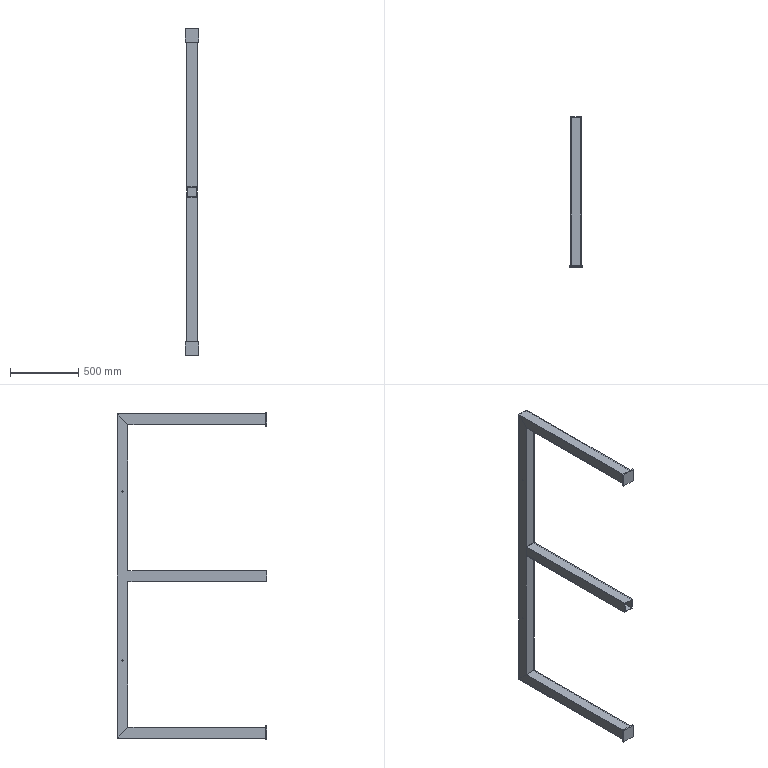Part | STEP file | Inner frame 1 | 1 solid | 55 faces | box 100 x 1100 x 2400 mm | volume 8328429 mm3 | plane 47 | cylinder 8 | commonest cylinder face diameters 10 x8
STEP:
#1=CARTESIAN_POINT('',(35.,1060.,-1775.5));
#2=VERTEX_POINT('',#1);
#3=CARTESIAN_POINT('',(35.,1060.,-1765.5));
#4=VERTEX_POINT('',#3);
#5=CARTESIAN_POINT('',(35.,1060.,-1770.5));
#6=DIRECTION('',(-1.,0.,0.));
#7=DIRECTION('',(0.,0.,1.));
#8=AXIS2_PLACEMENT_3D('',#5,#6,#7);
#9=CIRCLE('',#8,5.);
#10=EDGE_CURVE('',#2,#4,#9,.T.);
#11=ORIENTED_EDGE('',*,*,#10,.T.);
#12=CARTESIAN_POINT('',(40.,1060.,-1765.5));
#13=VERTEX_POINT('',#12);
#14=CARTESIAN_POINT('',(-50.,1060.,-1765.5));
#15=DIRECTION('',(1.,0.,0.));
#16=VECTOR('',#15,1000.);
#17=LINE('',#14,#16);
#18=EDGE_CURVE('',#4,#13,#17,.T.);
#19=ORIENTED_EDGE('',*,*,#18,.T.);
#20=CARTESIAN_POINT('',(40.,1060.,-1775.5));
#21=VERTEX_POINT('',#20);
#22=CARTESIAN_POINT('',(40.,1060.,-1770.5));
#23=DIRECTION('',(1.,0.,0.));
#24=DIRECTION('',(0.,0.,-1.));
#25=AXIS2_PLACEMENT_3D('',#22,#23,#24);
#26=CIRCLE('',#25,5.);
#27=EDGE_CURVE('',#13,#21,#26,.T.);
#28=ORIENTED_EDGE('',*,*,#27,.T.);
#29=CARTESIAN_POINT('',(-50.,1060.,-1775.5));
#30=DIRECTION('',(1.,0.,0.));
#31=VECTOR('',#30,1000.);
#32=LINE('',#29,#31);
#33=EDGE_CURVE('',#2,#21,#32,.T.);
#34=ORIENTED_EDGE('',*,*,#33,.F.);
#35=EDGE_LOOP('',(#11,#19,#28,#34));
#36=FACE_OUTER_BOUND('',#35,.T.);
#37=CARTESIAN_POINT('',(-50.,1060.,-1770.5));
#38=DIRECTION('',(1.,0.,0.));
#39=DIRECTION('',(0.,0.,-1.));
#40=AXIS2_PLACEMENT_3D('',#37,#38,#39);
#41=CYLINDRICAL_SURFACE('',#40,5.);
#42=ADVANCED_FACE('',(#36),#41,.F.);
#43=CARTESIAN_POINT('',(35.,1060.,-535.5));
#44=VERTEX_POINT('',#43);
#45=CARTESIAN_POINT('',(35.,1060.,-525.5));
#46=VERTEX_POINT('',#45);
#47=CARTESIAN_POINT('',(35.,1060.,-530.5));
#48=DIRECTION('',(-1.,0.,0.));
#49=DIRECTION('',(0.,0.,1.));
#50=AXIS2_PLACEMENT_3D('',#47,#48,#49);
#51=CIRCLE('',#50,5.);
#52=EDGE_CURVE('',#44,#46,#51,.T.);
#53=ORIENTED_EDGE('',*,*,#52,.T.);
#54=CARTESIAN_POINT('',(40.,1060.,-525.5));
#55=VERTEX_POINT('',#54);
#56=CARTESIAN_POINT('',(-50.,1060.,-525.5));
#57=DIRECTION('',(1.,0.,0.));
#58=VECTOR('',#57,1000.);
#59=LINE('',#56,#58);
#60=EDGE_CURVE('',#46,#55,#59,.T.);
#61=ORIENTED_EDGE('',*,*,#60,.T.);
#62=CARTESIAN_POINT('',(40.,1060.,-535.5));
#63=VERTEX_POINT('',#62);
#64=CARTESIAN_POINT('',(40.,1060.,-530.5));
#65=DIRECTION('',(1.,0.,0.));
#66=DIRECTION('',(0.,0.,-1.));
#67=AXIS2_PLACEMENT_3D('',#64,#65,#66);
#68=CIRCLE('',#67,5.);
#69=EDGE_CURVE('',#55,#63,#68,.T.);
#70=ORIENTED_EDGE('',*,*,#69,.T.);
#71=CARTESIAN_POINT('',(-50.,1060.,-535.5));
#72=DIRECTION('',(1.,0.,0.));
#73=VECTOR('',#72,1000.);
#74=LINE('',#71,#73);
#75=EDGE_CURVE('',#44,#63,#74,.T.);
#76=ORIENTED_EDGE('',*,*,#75,.F.);
#77=EDGE_LOOP('',(#53,#61,#70,#76));
#78=FACE_OUTER_BOUND('',#77,.T.);
#79=CARTESIAN_POINT('',(-50.,1060.,-530.5));
#80=DIRECTION('',(1.,0.,0.));
#81=DIRECTION('',(0.,0.,-1.));
#82=AXIS2_PLACEMENT_3D('',#79,#80,#81);
#83=CYLINDRICAL_SURFACE('',#82,5.);
#84=ADVANCED_FACE('',(#78),#83,.F.);
#85=CARTESIAN_POINT('',(-40.,1060.,-1775.5));
#86=VERTEX_POINT('',#85);
#87=CARTESIAN_POINT('',(-40.,1060.,-1765.5));
#88=VERTEX_POINT('',#87);
#89=CARTESIAN_POINT('',(-40.,1060.,-1770.5));
#90=DIRECTION('',(-1.,0.,0.));
#91=DIRECTION('',(0.,0.,1.));
#92=AXIS2_PLACEMENT_3D('',#89,#90,#91);
#93=CIRCLE('',#92,5.);
#94=EDGE_CURVE('',#86,#88,#93,.T.);
#95=ORIENTED_EDGE('',*,*,#94,.T.);
#96=CARTESIAN_POINT('',(-35.,1060.,-1765.5));
#97=VERTEX_POINT('',#96);
#98=CARTESIAN_POINT('',(-50.,1060.,-1765.5));
#99=DIRECTION('',(1.,0.,0.));
#100=VECTOR('',#99,1000.);
#101=LINE('',#98,#100);
#102=EDGE_CURVE('',#88,#97,#101,.T.);
#103=ORIENTED_EDGE('',*,*,#102,.T.);
#104=CARTESIAN_POINT('',(-35.,1060.,-1775.5));
#105=VERTEX_POINT('',#104);
#106=CARTESIAN_POINT('',(-35.,1060.,-1770.5));
#107=DIRECTION('',(1.,0.,0.));
#108=DIRECTION('',(0.,0.,-1.));
#109=AXIS2_PLACEMENT_3D('',#106,#107,#108);
#110=CIRCLE('',#109,5.);
#111=EDGE_CURVE('',#97,#105,#110,.T.);
#112=ORIENTED_EDGE('',*,*,#111,.T.);
#113=CARTESIAN_POINT('',(-50.,1060.,-1775.5));
#114=DIRECTION('',(1.,0.,0.));
#115=VECTOR('',#114,1000.);
#116=LINE('',#113,#115);
#117=EDGE_CURVE('',#86,#105,#116,.T.);
#118=ORIENTED_EDGE('',*,*,#117,.F.);
#119=EDGE_LOOP('',(#95,#103,#112,#118));
#120=FACE_OUTER_BOUND('',#119,.T.);
#121=CARTESIAN_POINT('',(-50.,1060.,-1770.5));
#122=DIRECTION('',(1.,0.,0.));
#123=DIRECTION('',(0.,0.,-1.));
#124=AXIS2_PLACEMENT_3D('',#121,#122,#123);
#125=CYLINDRICAL_SURFACE('',#124,5.);
#126=ADVANCED_FACE('',(#120),#125,.F.);
#127=CARTESIAN_POINT('',(-40.,1060.,-535.5));
#128=VERTEX_POINT('',#127);
#129=CARTESIAN_POINT('',(-40.,1060.,-525.5));
#130=VERTEX_POINT('',#129);
#131=CARTESIAN_POINT('',(-40.,1060.,-530.5));
#132=DIRECTION('',(-1.,0.,0.));
#133=DIRECTION('',(0.,0.,1.));
#134=AXIS2_PLACEMENT_3D('',#131,#132,#133);
#135=CIRCLE('',#134,5.);
#136=EDGE_CURVE('',#128,#130,#135,.T.);
#137=ORIENTED_EDGE('',*,*,#136,.T.);
#138=CARTESIAN_POINT('',(-35.,1060.,-525.5));
#139=VERTEX_POINT('',#138);
#140=CARTESIAN_POINT('',(-50.,1060.,-525.5));
#141=DIRECTION('',(1.,0.,0.));
#142=VECTOR('',#141,1000.);
#143=LINE('',#140,#142);
#144=EDGE_CURVE('',#130,#139,#143,.T.);
#145=ORIENTED_EDGE('',*,*,#144,.T.);
#146=CARTESIAN_POINT('',(-35.,1060.,-535.5));
#147=VERTEX_POINT('',#146);
#148=CARTESIAN_POINT('',(-35.,1060.,-530.5));
#149=DIRECTION('',(1.,0.,0.));
#150=DIRECTION('',(0.,0.,-1.));
#151=AXIS2_PLACEMENT_3D('',#148,#149,#150);
#152=CIRCLE('',#151,5.);
#153=EDGE_CURVE('',#139,#147,#152,.T.);
#154=ORIENTED_EDGE('',*,*,#153,.T.);
#155=CARTESIAN_POINT('',(-50.,1060.,-535.5));
#156=DIRECTION('',(1.,0.,0.));
#157=VECTOR('',#156,1000.);
#158=LINE('',#155,#157);
#159=EDGE_CURVE('',#128,#147,#158,.T.);
#160=ORIENTED_EDGE('',*,*,#159,.F.);
#161=EDGE_LOOP('',(#137,#145,#154,#160));
#162=FACE_OUTER_BOUND('',#161,.T.);
#163=CARTESIAN_POINT('',(-50.,1060.,-530.5));
#164=DIRECTION('',(1.,0.,0.));
#165=DIRECTION('',(0.,0.,-1.));
#166=AXIS2_PLACEMENT_3D('',#163,#164,#165);
#167=CYLINDRICAL_SURFACE('',#166,5.);
#168=ADVANCED_FACE('',(#162),#167,.F.);
#169=CARTESIAN_POINT('',(40.,1020.,-2260.));
#170=VERTEX_POINT('',#169);
#171=CARTESIAN_POINT('',(40.,10.,-2260.));
#172=VERTEX_POINT('',#171);
#173=CARTESIAN_POINT('',(40.,1104.1,-2260.));
#174=DIRECTION('',(0.,-1.,0.));
#175=VECTOR('',#174,1000.);
#176=LINE('',#173,#175);
#177=EDGE_CURVE('',#170,#172,#176,.T.);
#178=ORIENTED_EDGE('',*,*,#177,.T.);
#179=CARTESIAN_POINT('',(40.,10.,-2340.));
#180=VERTEX_POINT('',#179);
#181=CARTESIAN_POINT('',(40.,10.,-2340.));
#182=DIRECTION('',(0.,0.,-1.));
#183=VECTOR('',#182,1000.);
#184=LINE('',#181,#183);
#185=EDGE_CURVE('',#172,#180,#184,.T.);
#186=ORIENTED_EDGE('',*,*,#185,.T.);
#187=CARTESIAN_POINT('',(40.,1100.,-2340.));
#188=VERTEX_POINT('',#187);
#189=CARTESIAN_POINT('',(40.,1104.1,-2340.));
#190=DIRECTION('',(0.,-1.,0.));
#191=VECTOR('',#190,1000.);
#192=LINE('',#189,#191);
#193=EDGE_CURVE('',#188,#180,#192,.T.);
#194=ORIENTED_EDGE('',*,*,#193,.F.);
#195=CARTESIAN_POINT('',(40.,-92.05,-1147.95));
#196=DIRECTION('',(0.,0.7071,-0.7071));
#197=VECTOR('',#196,1000.);
#198=LINE('',#195,#197);
#199=EDGE_CURVE('',#170,#188,#198,.T.);
#200=ORIENTED_EDGE('',*,*,#199,.F.);
#201=EDGE_LOOP('',(#178,#186,#194,#200));
#202=FACE_OUTER_BOUND('',#201,.T.);
#203=CARTESIAN_POINT('',(40.,1104.1,-2340.));
#204=DIRECTION('',(1.,0.,0.));
#205=DIRECTION('',(0.,0.,-1.));
#206=AXIS2_PLACEMENT_3D('',#203,#204,#205);
#207=PLANE('',#206);
#208=ADVANCED_FACE('',(#202),#207,.T.);
#209=CARTESIAN_POINT('',(-40.,1020.,-2260.));
#210=VERTEX_POINT('',#209);
#211=CARTESIAN_POINT('',(-40.,10.,-2260.));
#212=VERTEX_POINT('',#211);
#213=CARTESIAN_POINT('',(-40.,1104.1,-2260.));
#214=DIRECTION('',(0.,-1.,0.));
#215=VECTOR('',#214,1000.);
#216=LINE('',#213,#215);
#217=EDGE_CURVE('',#210,#212,#216,.T.);
#218=ORIENTED_EDGE('',*,*,#217,.T.);
#219=CARTESIAN_POINT('',(40.,10.,-2260.));
#220=DIRECTION('',(1.,0.,0.));
#221=VECTOR('',#220,1000.);
#222=LINE('',#219,#221);
#223=EDGE_CURVE('',#212,#172,#222,.T.);
#224=ORIENTED_EDGE('',*,*,#223,.T.);
#225=ORIENTED_EDGE('',*,*,#177,.F.);
#226=CARTESIAN_POINT('',(40.,1020.,-2260.));
#227=DIRECTION('',(1.,0.,0.));
#228=VECTOR('',#227,1000.);
#229=LINE('',#226,#228);
#230=EDGE_CURVE('',#210,#170,#229,.T.);
#231=ORIENTED_EDGE('',*,*,#230,.F.);
#232=EDGE_LOOP('',(#218,#224,#225,#231));
#233=FACE_OUTER_BOUND('',#232,.T.);
#234=CARTESIAN_POINT('',(40.,1104.1,-2260.));
#235=DIRECTION('',(0.,0.,1.));
#236=DIRECTION('',(1.,0.,0.));
#237=AXIS2_PLACEMENT_3D('',#234,#235,#236);
#238=PLANE('',#237);
#239=ADVANCED_FACE('',(#233),#238,.T.);
#240=CARTESIAN_POINT('',(-40.,1100.,-2340.));
#241=VERTEX_POINT('',#240);
#242=CARTESIAN_POINT('',(-40.,10.,-2340.));
#243=VERTEX_POINT('',#242);
#244=CARTESIAN_POINT('',(-40.,1104.1,-2340.));
#245=DIRECTION('',(0.,-1.,0.));
#246=VECTOR('',#245,1000.);
#247=LINE('',#244,#246);
#248=EDGE_CURVE('',#241,#243,#247,.T.);
#249=ORIENTED_EDGE('',*,*,#248,.T.);
#250=CARTESIAN_POINT('',(-40.,10.,-2340.));
#251=DIRECTION('',(0.,0.,1.));
#252=VECTOR('',#251,1000.);
#253=LINE('',#250,#252);
#254=EDGE_CURVE('',#243,#212,#253,.T.);
#255=ORIENTED_EDGE('',*,*,#254,.T.);
#256=ORIENTED_EDGE('',*,*,#217,.F.);
#257=CARTESIAN_POINT('',(-40.,-92.05,-1147.95));
#258=DIRECTION('',(0.,-0.7071,0.7071));
#259=VECTOR('',#258,1000.);
#260=LINE('',#257,#259);
#261=EDGE_CURVE('',#241,#210,#260,.T.);
#262=ORIENTED_EDGE('',*,*,#261,.F.);
#263=EDGE_LOOP('',(#249,#255,#256,#262));
#264=FACE_OUTER_BOUND('',#263,.T.);
#265=CARTESIAN_POINT('',(-40.,1104.1,-2340.));
#266=DIRECTION('',(-1.,0.,0.));
#267=DIRECTION('',(0.,0.,1.));
#268=AXIS2_PLACEMENT_3D('',#265,#266,#267);
#269=PLANE('',#268);
#270=ADVANCED_FACE('',(#264),#269,.T.);
#271=ORIENTED_EDGE('',*,*,#193,.T.);
#272=CARTESIAN_POINT('',(40.,10.,-2340.));
#273=DIRECTION('',(-1.,0.,0.));
#274=VECTOR('',#273,1000.);
#275=LINE('',#272,#274);
#276=EDGE_CURVE('',#180,#243,#275,.T.);
#277=ORIENTED_EDGE('',*,*,#276,.T.);
#278=ORIENTED_EDGE('',*,*,#248,.F.);
#279=CARTESIAN_POINT('',(40.,1100.,-2340.));
#280=DIRECTION('',(-1.,0.,0.));
#281=VECTOR('',#280,1000.);
#282=LINE('',#279,#281);
#283=EDGE_CURVE('',#188,#241,#282,.T.);
#284=ORIENTED_EDGE('',*,*,#283,.F.);
#285=EDGE_LOOP('',(#271,#277,#278,#284));
#286=FACE_OUTER_BOUND('',#285,.T.);
#287=CARTESIAN_POINT('',(40.,1104.1,-2340.));
#288=DIRECTION('',(0.,0.,-1.));
#289=DIRECTION('',(-1.,0.,0.));
#290=AXIS2_PLACEMENT_3D('',#287,#288,#289);
#291=PLANE('',#290);
#292=ADVANCED_FACE('',(#286),#291,.T.);
#293=CARTESIAN_POINT('',(-40.,10.,40.));
#294=VERTEX_POINT('',#293);
#295=CARTESIAN_POINT('',(-40.,1100.,40.));
#296=VERTEX_POINT('',#295);
#297=CARTESIAN_POINT('',(-40.,0.,40.));
#298=DIRECTION('',(0.,1.,0.));
#299=VECTOR('',#298,1000.);
#300=LINE('',#297,#299);
#301=EDGE_CURVE('',#294,#296,#300,.T.);
#302=ORIENTED_EDGE('',*,*,#301,.F.);
#303=CARTESIAN_POINT('',(40.,10.,40.));
#304=VERTEX_POINT('',#303);
#305=CARTESIAN_POINT('',(40.,10.,40.));
#306=DIRECTION('',(1.,0.,0.));
#307=VECTOR('',#306,1000.);
#308=LINE('',#305,#307);
#309=EDGE_CURVE('',#294,#304,#308,.T.);
#310=ORIENTED_EDGE('',*,*,#309,.T.);
#311=CARTESIAN_POINT('',(40.,1100.,40.));
#312=VERTEX_POINT('',#311);
#313=CARTESIAN_POINT('',(40.,0.,40.));
#314=DIRECTION('',(0.,1.,0.));
#315=VECTOR('',#314,1000.);
#316=LINE('',#313,#315);
#317=EDGE_CURVE('',#304,#312,#316,.T.);
#318=ORIENTED_EDGE('',*,*,#317,.T.);
#319=CARTESIAN_POINT('',(40.,1100.,40.));
#320=DIRECTION('',(-1.,0.,0.));
#321=VECTOR('',#320,1000.);
#322=LINE('',#319,#321);
#323=EDGE_CURVE('',#312,#296,#322,.T.);
#324=ORIENTED_EDGE('',*,*,#323,.T.);
#325=EDGE_LOOP('',(#302,#310,#318,#324));
#326=FACE_OUTER_BOUND('',#325,.T.);
#327=CARTESIAN_POINT('',(40.,0.,40.));
#328=DIRECTION('',(0.,0.,1.));
#329=DIRECTION('',(1.,0.,0.));
#330=AXIS2_PLACEMENT_3D('',#327,#328,#329);
#331=PLANE('',#330);
#332=ADVANCED_FACE('',(#326),#331,.T.);
#333=CARTESIAN_POINT('',(-40.,10.,-40.));
#334=VERTEX_POINT('',#333);
#335=CARTESIAN_POINT('',(-40.,1020.,-40.));
#336=VERTEX_POINT('',#335);
#337=CARTESIAN_POINT('',(-40.,0.,-40.));
#338=DIRECTION('',(0.,1.,0.));
#339=VECTOR('',#338,1000.);
#340=LINE('',#337,#339);
#341=EDGE_CURVE('',#334,#336,#340,.T.);
#342=ORIENTED_EDGE('',*,*,#341,.F.);
#343=CARTESIAN_POINT('',(-40.,10.,40.));
#344=DIRECTION('',(0.,0.,1.));
#345=VECTOR('',#344,1000.);
#346=LINE('',#343,#345);
#347=EDGE_CURVE('',#334,#294,#346,.T.);
#348=ORIENTED_EDGE('',*,*,#347,.T.);
#349=ORIENTED_EDGE('',*,*,#301,.T.);
#350=CARTESIAN_POINT('',(-40.,550.,-510.));
#351=DIRECTION('',(0.,-0.7071,-0.7071));
#352=VECTOR('',#351,1000.);
#353=LINE('',#350,#352);
#354=EDGE_CURVE('',#296,#336,#353,.T.);
#355=ORIENTED_EDGE('',*,*,#354,.T.);
#356=EDGE_LOOP('',(#342,#348,#349,#355));
#357=FACE_OUTER_BOUND('',#356,.T.);
#358=CARTESIAN_POINT('',(-40.,0.,40.));
#359=DIRECTION('',(-1.,0.,0.));
#360=DIRECTION('',(0.,0.,1.));
#361=AXIS2_PLACEMENT_3D('',#358,#359,#360);
#362=PLANE('',#361);
#363=ADVANCED_FACE('',(#357),#362,.T.);
#364=CARTESIAN_POINT('',(40.,10.,-40.));
#365=VERTEX_POINT('',#364);
#366=CARTESIAN_POINT('',(40.,1020.,-40.));
#367=VERTEX_POINT('',#366);
#368=CARTESIAN_POINT('',(40.,0.,-40.));
#369=DIRECTION('',(0.,1.,0.));
#370=VECTOR('',#369,1000.);
#371=LINE('',#368,#370);
#372=EDGE_CURVE('',#365,#367,#371,.T.);
#373=ORIENTED_EDGE('',*,*,#372,.F.);
#374=CARTESIAN_POINT('',(40.,10.,-40.));
#375=DIRECTION('',(-1.,0.,0.));
#376=VECTOR('',#375,1000.);
#377=LINE('',#374,#376);
#378=EDGE_CURVE('',#365,#334,#377,.T.);
#379=ORIENTED_EDGE('',*,*,#378,.T.);
#380=ORIENTED_EDGE('',*,*,#341,.T.);
#381=CARTESIAN_POINT('',(40.,1020.,-40.));
#382=DIRECTION('',(1.,0.,0.));
#383=VECTOR('',#382,1000.);
#384=LINE('',#381,#383);
#385=EDGE_CURVE('',#336,#367,#384,.T.);
#386=ORIENTED_EDGE('',*,*,#385,.T.);
#387=EDGE_LOOP('',(#373,#379,#380,#386));
#388=FACE_OUTER_BOUND('',#387,.T.);
#389=CARTESIAN_POINT('',(40.,0.,-40.));
#390=DIRECTION('',(0.,0.,-1.));
#391=DIRECTION('',(-1.,0.,0.));
#392=AXIS2_PLACEMENT_3D('',#389,#390,#391);
#393=PLANE('',#392);
#394=ADVANCED_FACE('',(#388),#393,.T.);
#395=ORIENTED_EDGE('',*,*,#317,.F.);
#396=CARTESIAN_POINT('',(40.,10.,40.));
#397=DIRECTION('',(0.,0.,-1.));
#398=VECTOR('',#397,1000.);
#399=LINE('',#396,#398);
#400=EDGE_CURVE('',#304,#365,#399,.T.);
#401=ORIENTED_EDGE('',*,*,#400,.T.);
#402=ORIENTED_EDGE('',*,*,#372,.T.);
#403=CARTESIAN_POINT('',(40.,550.,-510.));
#404=DIRECTION('',(0.,0.7071,0.7071));
#405=VECTOR('',#404,1000.);
#406=LINE('',#403,#405);
#407=EDGE_CURVE('',#367,#312,#406,.T.);
#408=ORIENTED_EDGE('',*,*,#407,.T.);
#409=EDGE_LOOP('',(#395,#401,#402,#408));
#410=FACE_OUTER_BOUND('',#409,.T.);
#411=CARTESIAN_POINT('',(40.,0.,40.));
#412=DIRECTION('',(1.,0.,0.));
#413=DIRECTION('',(0.,0.,-1.));
#414=AXIS2_PLACEMENT_3D('',#411,#412,#413);
#415=PLANE('',#414);
#416=ADVANCED_FACE('',(#410),#415,.T.);
#417=CARTESIAN_POINT('',(40.,1020.,-1190.5));
#418=VERTEX_POINT('',#417);
#419=CARTESIAN_POINT('',(40.,1020.,44.1));
#420=DIRECTION('',(0.,0.,-1.));
#421=VECTOR('',#420,1000.);
#422=LINE('',#419,#421);
#423=EDGE_CURVE('',#418,#170,#422,.T.);
#424=ORIENTED_EDGE('',*,*,#423,.F.);
#425=CARTESIAN_POINT('',(-40.,1020.,-1190.5));
#426=VERTEX_POINT('',#425);
#427=CARTESIAN_POINT('',(-40.,1020.,-1190.5));
#428=DIRECTION('',(1.,0.,0.));
#429=VECTOR('',#428,1000.);
#430=LINE('',#427,#429);
#431=EDGE_CURVE('',#426,#418,#430,.T.);
#432=ORIENTED_EDGE('',*,*,#431,.F.);
#433=CARTESIAN_POINT('',(-40.,1020.,44.1));
#434=DIRECTION('',(0.,0.,-1.));
#435=VECTOR('',#434,1000.);
#436=LINE('',#433,#435);
#437=EDGE_CURVE('',#426,#210,#436,.T.);
#438=ORIENTED_EDGE('',*,*,#437,.T.);
#439=ORIENTED_EDGE('',*,*,#230,.T.);
#440=EDGE_LOOP('',(#424,#432,#438,#439));
#441=FACE_OUTER_BOUND('',#440,.T.);
#442=CARTESIAN_POINT('',(40.,1020.,44.1));
#443=DIRECTION('',(0.,-1.,0.));
#444=DIRECTION('',(1.,0.,0.));
#445=AXIS2_PLACEMENT_3D('',#442,#443,#444);
#446=PLANE('',#445);
#447=ADVANCED_FACE('',(#441),#446,.T.);
#448=CARTESIAN_POINT('',(-40.,1020.,-1110.5));
#449=VERTEX_POINT('',#448);
#450=CARTESIAN_POINT('',(-40.,1020.,44.1));
#451=DIRECTION('',(0.,0.,-1.));
#452=VECTOR('',#451,1000.);
#453=LINE('',#450,#452);
#454=EDGE_CURVE('',#336,#449,#453,.T.);
#455=ORIENTED_EDGE('',*,*,#454,.T.);
#456=CARTESIAN_POINT('',(40.,1020.,-1110.5));
#457=VERTEX_POINT('',#456);
#458=CARTESIAN_POINT('',(-40.,1020.,-1110.5));
#459=DIRECTION('',(-1.,0.,0.));
#460=VECTOR('',#459,1000.);
#461=LINE('',#458,#460);
#462=EDGE_CURVE('',#457,#449,#461,.T.);
#463=ORIENTED_EDGE('',*,*,#462,.F.);
#464=CARTESIAN_POINT('',(40.,1020.,44.1));
#465=DIRECTION('',(0.,0.,-1.));
#466=VECTOR('',#465,1000.);
#467=LINE('',#464,#466);
#468=EDGE_CURVE('',#367,#457,#467,.T.);
#469=ORIENTED_EDGE('',*,*,#468,.F.);
#470=ORIENTED_EDGE('',*,*,#385,.F.);
#471=EDGE_LOOP('',(#455,#463,#469,#470));
#472=FACE_OUTER_BOUND('',#471,.T.);
#473=CARTESIAN_POINT('',(40.,1020.,44.1));
#474=DIRECTION('',(0.,-1.,0.));
#475=DIRECTION('',(1.,0.,0.));
#476=AXIS2_PLACEMENT_3D('',#473,#474,#475);
#477=PLANE('',#476);
#478=ADVANCED_FACE('',(#472),#477,.T.);
#479=CARTESIAN_POINT('',(40.,1060.,-1770.5));
#480=DIRECTION('',(1.,0.,0.));
#481=DIRECTION('',(0.,0.,-1.));
#482=AXIS2_PLACEMENT_3D('',#479,#480,#481);
#483=CIRCLE('',#482,5.);
#484=EDGE_CURVE('',#21,#13,#483,.T.);
#485=ORIENTED_EDGE('',*,*,#484,.F.);
#486=ORIENTED_EDGE('',*,*,#27,.F.);
#487=EDGE_LOOP('',(#485,#486));
#488=FACE_BOUND('',#487,.T.);
#489=CARTESIAN_POINT('',(40.,1060.,-530.5));
#490=DIRECTION('',(1.,0.,0.));
#491=DIRECTION('',(0.,0.,-1.));
#492=AXIS2_PLACEMENT_3D('',#489,#490,#491);
#493=CIRCLE('',#492,5.);
#494=EDGE_CURVE('',#63,#55,#493,.T.);
#495=ORIENTED_EDGE('',*,*,#494,.F.);
#496=ORIENTED_EDGE('',*,*,#69,.F.);
#497=EDGE_LOOP('',(#495,#496));
#498=FACE_BOUND('',#497,.T.);
#499=CARTESIAN_POINT('',(40.,0.,-1190.5));
#500=VERTEX_POINT('',#499);
#501=CARTESIAN_POINT('',(40.,-113.137,-1190.5));
#502=DIRECTION('',(0.,1.,0.));
#503=VECTOR('',#502,1000.);
#504=LINE('',#501,#503);
#505=EDGE_CURVE('',#500,#418,#504,.T.);
#506=ORIENTED_EDGE('',*,*,#505,.T.);
#507=ORIENTED_EDGE('',*,*,#423,.T.);
#508=ORIENTED_EDGE('',*,*,#199,.T.);
#509=CARTESIAN_POINT('',(40.,1100.,44.1));
#510=DIRECTION('',(0.,0.,-1.));
#511=VECTOR('',#510,1000.);
#512=LINE('',#509,#511);
#513=EDGE_CURVE('',#312,#188,#512,.T.);
#514=ORIENTED_EDGE('',*,*,#513,.F.);
#515=ORIENTED_EDGE('',*,*,#407,.F.);
#516=ORIENTED_EDGE('',*,*,#468,.T.);
#517=CARTESIAN_POINT('',(40.,0.,-1110.5));
#518=VERTEX_POINT('',#517);
#519=CARTESIAN_POINT('',(40.,-113.137,-1110.5));
#520=DIRECTION('',(0.,1.,0.));
#521=VECTOR('',#520,1000.);
#522=LINE('',#519,#521);
#523=EDGE_CURVE('',#518,#457,#522,.T.);
#524=ORIENTED_EDGE('',*,*,#523,.F.);
#525=CARTESIAN_POINT('',(40.,0.,-1110.5));
#526=DIRECTION('',(0.,0.,1.));
#527=VECTOR('',#526,1000.);
#528=LINE('',#525,#527);
#529=EDGE_CURVE('',#500,#518,#528,.T.);
#530=ORIENTED_EDGE('',*,*,#529,.F.);
#531=EDGE_LOOP('',(#506,#507,#508,#514,#515,#516,#524,#530));
#532=FACE_OUTER_BOUND('',#531,.T.);
#533=CARTESIAN_POINT('',(40.,1100.,44.1));
#534=DIRECTION('',(1.,0.,0.));
#535=DIRECTION('',(0.,0.,-1.));
#536=AXIS2_PLACEMENT_3D('',#533,#534,#535);
#537=PLANE('',#536);
#538=ADVANCED_FACE('',(#488,#498,#532),#537,.T.);
#539=ORIENTED_EDGE('',*,*,#94,.F.);
#540=CARTESIAN_POINT('',(-40.,1060.,-1770.5));
#541=DIRECTION('',(-1.,0.,0.));
#542=DIRECTION('',(0.,0.,1.));
#543=AXIS2_PLACEMENT_3D('',#540,#541,#542);
#544=CIRCLE('',#543,5.);
#545=EDGE_CURVE('',#88,#86,#544,.T.);
#546=ORIENTED_EDGE('',*,*,#545,.F.);
#547=EDGE_LOOP('',(#539,#546));
#548=FACE_BOUND('',#547,.T.);
#549=ORIENTED_EDGE('',*,*,#136,.F.);
#550=CARTESIAN_POINT('',(-40.,1060.,-530.5));
#551=DIRECTION('',(-1.,0.,0.));
#552=DIRECTION('',(0.,0.,1.));
#553=AXIS2_PLACEMENT_3D('',#550,#551,#552);
#554=CIRCLE('',#553,5.);
#555=EDGE_CURVE('',#130,#128,#554,.T.);
#556=ORIENTED_EDGE('',*,*,#555,.F.);
#557=EDGE_LOOP('',(#549,#556));
#558=FACE_BOUND('',#557,.T.);
#559=CARTESIAN_POINT('',(-40.,0.,-1110.5));
#560=VERTEX_POINT('',#559);
#561=CARTESIAN_POINT('',(-40.,-113.137,-1110.5));
#562=DIRECTION('',(0.,1.,0.));
#563=VECTOR('',#562,1000.);
#564=LINE('',#561,#563);
#565=EDGE_CURVE('',#560,#449,#564,.T.);
#566=ORIENTED_EDGE('',*,*,#565,.T.);
#567=ORIENTED_EDGE('',*,*,#454,.F.);
#568=ORIENTED_EDGE('',*,*,#354,.F.);
#569=CARTESIAN_POINT('',(-40.,1100.,44.1));
#570=DIRECTION('',(0.,0.,-1.));
#571=VECTOR('',#570,1000.);
#572=LINE('',#569,#571);
#573=EDGE_CURVE('',#296,#241,#572,.T.);
#574=ORIENTED_EDGE('',*,*,#573,.T.);
#575=ORIENTED_EDGE('',*,*,#261,.T.);
#576=ORIENTED_EDGE('',*,*,#437,.F.);
#577=CARTESIAN_POINT('',(-40.,0.,-1190.5));
#578=VERTEX_POINT('',#577);
#579=CARTESIAN_POINT('',(-40.,-113.137,-1190.5));
#580=DIRECTION('',(0.,1.,0.));
#581=VECTOR('',#580,1000.);
#582=LINE('',#579,#581);
#583=EDGE_CURVE('',#578,#426,#582,.T.);
#584=ORIENTED_EDGE('',*,*,#583,.F.);
#585=CARTESIAN_POINT('',(-40.,0.,-1110.5));
#586=DIRECTION('',(0.,0.,-1.));
#587=VECTOR('',#586,1000.);
#588=LINE('',#585,#587);
#589=EDGE_CURVE('',#560,#578,#588,.T.);
#590=ORIENTED_EDGE('',*,*,#589,.F.);
#591=EDGE_LOOP('',(#566,#567,#568,#574,#575,#576,#584,#590));
#592=FACE_OUTER_BOUND('',#591,.T.);
#593=CARTESIAN_POINT('',(-40.,1100.,44.1));
#594=DIRECTION('',(-1.,0.,0.));
#595=DIRECTION('',(0.,0.,1.));
#596=AXIS2_PLACEMENT_3D('',#593,#594,#595);
#597=PLANE('',#596);
#598=ADVANCED_FACE('',(#548,#558,#592),#597,.T.);
#599=ORIENTED_EDGE('',*,*,#513,.T.);
#600=ORIENTED_EDGE('',*,*,#283,.T.);
#601=ORIENTED_EDGE('',*,*,#573,.F.);
#602=ORIENTED_EDGE('',*,*,#323,.F.);
#603=EDGE_LOOP('',(#599,#600,#601,#602));
#604=FACE_OUTER_BOUND('',#603,.T.);
#605=CARTESIAN_POINT('',(40.,1100.,44.1));
#606=DIRECTION('',(0.,1.,0.));
#607=DIRECTION('',(-1.,0.,0.));
#608=AXIS2_PLACEMENT_3D('',#605,#606,#607);
#609=PLANE('',#608);
#610=ADVANCED_FACE('',(#604),#609,.T.);
#611=ORIENTED_EDGE('',*,*,#583,.T.);
#612=ORIENTED_EDGE('',*,*,#431,.T.);
#613=ORIENTED_EDGE('',*,*,#505,.F.);
#614=CARTESIAN_POINT('',(-40.,0.,-1190.5));
#615=DIRECTION('',(1.,0.,0.));
#616=VECTOR('',#615,1000.);
#617=LINE('',#614,#616);
#618=EDGE_CURVE('',#578,#500,#617,.T.);
#619=ORIENTED_EDGE('',*,*,#618,.F.);
#620=EDGE_LOOP('',(#611,#612,#613,#619));
#621=FACE_OUTER_BOUND('',#620,.T.);
#622=CARTESIAN_POINT('',(-40.,-113.137,-1190.5));
#623=DIRECTION('',(0.,0.,1.));
#624=DIRECTION('',(1.,0.,0.));
#625=AXIS2_PLACEMENT_3D('',#622,#623,#624);
#626=PLANE('',#625);
#627=ADVANCED_FACE('',(#621),#626,.F.);
#628=ORIENTED_EDGE('',*,*,#523,.T.);
#629=ORIENTED_EDGE('',*,*,#462,.T.);
#630=ORIENTED_EDGE('',*,*,#565,.F.);
#631=CARTESIAN_POINT('',(-40.,0.,-1110.5));
#632=DIRECTION('',(-1.,0.,0.));
#633=VECTOR('',#632,1000.);
#634=LINE('',#631,#633);
#635=EDGE_CURVE('',#518,#560,#634,.T.);
#636=ORIENTED_EDGE('',*,*,#635,.F.);
#637=EDGE_LOOP('',(#628,#629,#630,#636));
#638=FACE_OUTER_BOUND('',#637,.T.);
#639=CARTESIAN_POINT('',(-40.,-113.137,-1110.5));
#640=DIRECTION('',(0.,0.,-1.));
#641=DIRECTION('',(-1.,0.,0.));
#642=AXIS2_PLACEMENT_3D('',#639,#640,#641);
#643=PLANE('',#642);
#644=ADVANCED_FACE('',(#638),#643,.F.);
#645=CARTESIAN_POINT('',(-35.,0.,-1115.5));
#646=VERTEX_POINT('',#645);
#647=CARTESIAN_POINT('',(-35.,1020.,-1115.5));
#648=VERTEX_POINT('',#647);
#649=CARTESIAN_POINT('',(-35.,-113.137,-1115.5));
#650=DIRECTION('',(0.,1.,0.));
#651=VECTOR('',#650,1000.);
#652=LINE('',#649,#651);
#653=EDGE_CURVE('',#646,#648,#652,.T.);
#654=ORIENTED_EDGE('',*,*,#653,.T.);
#655=CARTESIAN_POINT('',(35.,1020.,-1115.5));
#656=VERTEX_POINT('',#655);
#657=CARTESIAN_POINT('',(35.,1020.,-1115.5));
#658=DIRECTION('',(-1.,0.,0.));
#659=VECTOR('',#658,1000.);
#660=LINE('',#657,#659);
#661=EDGE_CURVE('',#656,#648,#660,.T.);
#662=ORIENTED_EDGE('',*,*,#661,.F.);
#663=CARTESIAN_POINT('',(35.,0.,-1115.5));
#664=VERTEX_POINT('',#663);
#665=CARTESIAN_POINT('',(35.,-113.137,-1115.5));
#666=DIRECTION('',(0.,1.,0.));
#667=VECTOR('',#666,1000.);
#668=LINE('',#665,#667);
#669=EDGE_CURVE('',#664,#656,#668,.T.);
#670=ORIENTED_EDGE('',*,*,#669,.F.);
#671=CARTESIAN_POINT('',(35.,0.,-1115.5));
#672=DIRECTION('',(-1.,0.,0.));
#673=VECTOR('',#672,1000.);
#674=LINE('',#671,#673);
#675=EDGE_CURVE('',#664,#646,#674,.T.);
#676=ORIENTED_EDGE('',*,*,#675,.T.);
#677=EDGE_LOOP('',(#654,#662,#670,#676));
#678=FACE_OUTER_BOUND('',#677,.T.);
#679=CARTESIAN_POINT('',(35.,-113.137,-1115.5));
#680=DIRECTION('',(0.,0.,-1.));
#681=DIRECTION('',(-1.,0.,0.));
#682=AXIS2_PLACEMENT_3D('',#679,#680,#681);
#683=PLANE('',#682);
#684=ADVANCED_FACE('',(#678),#683,.T.);
#685=ORIENTED_EDGE('',*,*,#669,.T.);
#686=CARTESIAN_POINT('',(35.,1020.,-1185.5));
#687=VERTEX_POINT('',#686);
#688=CARTESIAN_POINT('',(35.,1020.,-1185.5));
#689=DIRECTION('',(0.,0.,1.));
#690=VECTOR('',#689,1000.);
#691=LINE('',#688,#690);
#692=EDGE_CURVE('',#687,#656,#691,.T.);
#693=ORIENTED_EDGE('',*,*,#692,.F.);
#694=CARTESIAN_POINT('',(35.,0.,-1185.5));
#695=VERTEX_POINT('',#694);
#696=CARTESIAN_POINT('',(35.,-113.137,-1185.5));
#697=DIRECTION('',(0.,1.,0.));
#698=VECTOR('',#697,1000.);
#699=LINE('',#696,#698);
#700=EDGE_CURVE('',#695,#687,#699,.T.);
#701=ORIENTED_EDGE('',*,*,#700,.F.);
#702=CARTESIAN_POINT('',(35.,0.,-1185.5));
#703=DIRECTION('',(0.,0.,1.));
#704=VECTOR('',#703,1000.);
#705=LINE('',#702,#704);
#706=EDGE_CURVE('',#695,#664,#705,.T.);
#707=ORIENTED_EDGE('',*,*,#706,.T.);
#708=EDGE_LOOP('',(#685,#693,#701,#707));
#709=FACE_OUTER_BOUND('',#708,.T.);
#710=CARTESIAN_POINT('',(35.,-113.137,-1185.5));
#711=DIRECTION('',(-1.,0.,0.));
#712=DIRECTION('',(0.,-1.,0.));
#713=AXIS2_PLACEMENT_3D('',#710,#711,#712);
#714=PLANE('',#713);
#715=ADVANCED_FACE('',(#709),#714,.T.);
#716=ORIENTED_EDGE('',*,*,#700,.T.);
#717=CARTESIAN_POINT('',(-35.,1020.,-1185.5));
#718=VERTEX_POINT('',#717);
#719=CARTESIAN_POINT('',(35.,1020.,-1185.5));
#720=DIRECTION('',(1.,0.,0.));
#721=VECTOR('',#720,1000.);
#722=LINE('',#719,#721);
#723=EDGE_CURVE('',#718,#687,#722,.T.);
#724=ORIENTED_EDGE('',*,*,#723,.F.);
#725=CARTESIAN_POINT('',(-35.,0.,-1185.5));
#726=VERTEX_POINT('',#725);
#727=CARTESIAN_POINT('',(-35.,-113.137,-1185.5));
#728=DIRECTION('',(0.,1.,0.));
#729=VECTOR('',#728,1000.);
#730=LINE('',#727,#729);
#731=EDGE_CURVE('',#726,#718,#730,.T.);
#732=ORIENTED_EDGE('',*,*,#731,.F.);
#733=CARTESIAN_POINT('',(35.,0.,-1185.5));
#734=DIRECTION('',(1.,0.,0.));
#735=VECTOR('',#734,1000.);
#736=LINE('',#733,#735);
#737=EDGE_CURVE('',#726,#695,#736,.T.);
#738=ORIENTED_EDGE('',*,*,#737,.T.);
#739=EDGE_LOOP('',(#716,#724,#732,#738));
#740=FACE_OUTER_BOUND('',#739,.T.);
#741=CARTESIAN_POINT('',(35.,-113.137,-1185.5));
#742=DIRECTION('',(0.,0.,1.));
#743=DIRECTION('',(1.,0.,0.));
#744=AXIS2_PLACEMENT_3D('',#741,#742,#743);
#745=PLANE('',#744);
#746=ADVANCED_FACE('',(#740),#745,.T.);
#747=ORIENTED_EDGE('',*,*,#731,.T.);
#748=CARTESIAN_POINT('',(-35.,1020.,-1185.5));
#749=DIRECTION('',(0.,0.,-1.));
#750=VECTOR('',#749,1000.);
#751=LINE('',#748,#750);
#752=EDGE_CURVE('',#648,#718,#751,.T.);
#753=ORIENTED_EDGE('',*,*,#752,.F.);
#754=ORIENTED_EDGE('',*,*,#653,.F.);
#755=CARTESIAN_POINT('',(-35.,0.,-1185.5));
#756=DIRECTION('',(0.,0.,-1.));
#757=VECTOR('',#756,1000.);
#758=LINE('',#755,#757);
#759=EDGE_CURVE('',#646,#726,#758,.T.);
#760=ORIENTED_EDGE('',*,*,#759,.T.);
#761=EDGE_LOOP('',(#747,#753,#754,#760));
#762=FACE_OUTER_BOUND('',#761,.T.);
#763=CARTESIAN_POINT('',(-35.,-113.137,-1185.5));
#764=DIRECTION('',(1.,0.,0.));
#765=DIRECTION('',(0.,1.,0.));
#766=AXIS2_PLACEMENT_3D('',#763,#764,#765);
#767=PLANE('',#766);
#768=ADVANCED_FACE('',(#762),#767,.T.);
#769=ORIENTED_EDGE('',*,*,#759,.F.);
#770=ORIENTED_EDGE('',*,*,#675,.F.);
#771=ORIENTED_EDGE('',*,*,#706,.F.);
#772=ORIENTED_EDGE('',*,*,#737,.F.);
#773=EDGE_LOOP('',(#769,#770,#771,#772));
#774=FACE_BOUND('',#773,.T.);
#775=ORIENTED_EDGE('',*,*,#618,.T.);
#776=ORIENTED_EDGE('',*,*,#529,.T.);
#777=ORIENTED_EDGE('',*,*,#635,.T.);
#778=ORIENTED_EDGE('',*,*,#589,.T.);
#779=EDGE_LOOP('',(#775,#776,#777,#778));
#780=FACE_OUTER_BOUND('',#779,.T.);
#781=CARTESIAN_POINT('',(0.,0.,-2300.));
#782=DIRECTION('',(0.,-1.,0.));
#783=DIRECTION('',(0.,0.,-1.));
#784=AXIS2_PLACEMENT_3D('',#781,#782,#783);
#785=PLANE('',#784);
#786=ADVANCED_FACE('',(#774,#780),#785,.T.);
#787=ORIENTED_EDGE('',*,*,#661,.T.);
#788=ORIENTED_EDGE('',*,*,#752,.T.);
#789=ORIENTED_EDGE('',*,*,#723,.T.);
#790=ORIENTED_EDGE('',*,*,#692,.T.);
#791=EDGE_LOOP('',(#787,#788,#789,#790));
#792=FACE_OUTER_BOUND('',#791,.T.);
#793=CARTESIAN_POINT('',(40.,1020.,44.1));
#794=DIRECTION('',(0.,-1.,0.));
#795=DIRECTION('',(1.,0.,0.));
#796=AXIS2_PLACEMENT_3D('',#793,#794,#795);
#797=PLANE('',#796);
#798=ADVANCED_FACE('',(#792),#797,.T.);
#799=ORIENTED_EDGE('',*,*,#309,.F.);
#800=ORIENTED_EDGE('',*,*,#347,.F.);
#801=ORIENTED_EDGE('',*,*,#378,.F.);
#802=ORIENTED_EDGE('',*,*,#400,.F.);
#803=EDGE_LOOP('',(#799,#800,#801,#802));
#804=FACE_BOUND('',#803,.T.);
#805=CARTESIAN_POINT('',(-50.,10.,50.));
#806=VERTEX_POINT('',#805);
#807=CARTESIAN_POINT('',(-50.,10.,-50.));
#808=VERTEX_POINT('',#807);
#809=CARTESIAN_POINT('',(-50.,10.,-50.));
#810=DIRECTION('',(0.,0.,-1.));
#811=VECTOR('',#810,1000.);
#812=LINE('',#809,#811);
#813=EDGE_CURVE('',#806,#808,#812,.T.);
#814=ORIENTED_EDGE('',*,*,#813,.F.);
#815=CARTESIAN_POINT('',(50.,10.,50.));
#816=VERTEX_POINT('',#815);
#817=CARTESIAN_POINT('',(50.,10.,50.));
#818=DIRECTION('',(-1.,0.,0.));
#819=VECTOR('',#818,1000.);
#820=LINE('',#817,#819);
#821=EDGE_CURVE('',#816,#806,#820,.T.);
#822=ORIENTED_EDGE('',*,*,#821,.F.);
#823=CARTESIAN_POINT('',(50.,10.,-50.));
#824=VERTEX_POINT('',#823);
#825=CARTESIAN_POINT('',(50.,10.,-50.));
#826=DIRECTION('',(0.,0.,1.));
#827=VECTOR('',#826,1000.);
#828=LINE('',#825,#827);
#829=EDGE_CURVE('',#824,#816,#828,.T.);
#830=ORIENTED_EDGE('',*,*,#829,.F.);
#831=CARTESIAN_POINT('',(50.,10.,-50.));
#832=DIRECTION('',(1.,0.,0.));
#833=VECTOR('',#832,1000.);
#834=LINE('',#831,#833);
#835=EDGE_CURVE('',#808,#824,#834,.T.);
#836=ORIENTED_EDGE('',*,*,#835,.F.);
#837=EDGE_LOOP('',(#814,#822,#830,#836));
#838=FACE_OUTER_BOUND('',#837,.T.);
#839=CARTESIAN_POINT('',(0.,10.,0.));
#840=DIRECTION('',(0.,-1.,0.));
#841=DIRECTION('',(0.,0.,-1.));
#842=AXIS2_PLACEMENT_3D('',#839,#840,#841);
#843=PLANE('',#842);
#844=ADVANCED_FACE('',(#804,#838),#843,.F.);
#845=CARTESIAN_POINT('',(-50.,0.,50.));
#846=VERTEX_POINT('',#845);
#847=CARTESIAN_POINT('',(-50.,0.,-50.));
#848=VERTEX_POINT('',#847);
#849=CARTESIAN_POINT('',(-50.,0.,-50.));
#850=DIRECTION('',(0.,0.,-1.));
#851=VECTOR('',#850,1000.);
#852=LINE('',#849,#851);
#853=EDGE_CURVE('',#846,#848,#852,.T.);
#854=ORIENTED_EDGE('',*,*,#853,.F.);
#855=CARTESIAN_POINT('',(-50.,10.,50.));
#856=DIRECTION('',(0.,-1.,0.));
#857=VECTOR('',#856,1000.);
#858=LINE('',#855,#857);
#859=EDGE_CURVE('',#806,#846,#858,.T.);
#860=ORIENTED_EDGE('',*,*,#859,.F.);
#861=ORIENTED_EDGE('',*,*,#813,.T.);
#862=CARTESIAN_POINT('',(-50.,10.,-50.));
#863=DIRECTION('',(0.,-1.,0.));
#864=VECTOR('',#863,1000.);
#865=LINE('',#862,#864);
#866=EDGE_CURVE('',#808,#848,#865,.T.);
#867=ORIENTED_EDGE('',*,*,#866,.T.);
#868=EDGE_LOOP('',(#854,#860,#861,#867));
#869=FACE_OUTER_BOUND('',#868,.T.);
#870=CARTESIAN_POINT('',(-50.,10.,-50.));
#871=DIRECTION('',(-1.,0.,0.));
#872=DIRECTION('',(0.,0.,1.));
#873=AXIS2_PLACEMENT_3D('',#870,#871,#872);
#874=PLANE('',#873);
#875=ADVANCED_FACE('',(#869),#874,.T.);
#876=CARTESIAN_POINT('',(50.,0.,50.));
#877=VERTEX_POINT('',#876);
#878=CARTESIAN_POINT('',(50.,0.,50.));
#879=DIRECTION('',(-1.,0.,0.));
#880=VECTOR('',#879,1000.);
#881=LINE('',#878,#880);
#882=EDGE_CURVE('',#877,#846,#881,.T.);
#883=ORIENTED_EDGE('',*,*,#882,.F.);
#884=CARTESIAN_POINT('',(50.,10.,50.));
#885=DIRECTION('',(0.,-1.,0.));
#886=VECTOR('',#885,1000.);
#887=LINE('',#884,#886);
#888=EDGE_CURVE('',#816,#877,#887,.T.);
#889=ORIENTED_EDGE('',*,*,#888,.F.);
#890=ORIENTED_EDGE('',*,*,#821,.T.);
#891=ORIENTED_EDGE('',*,*,#859,.T.);
#892=EDGE_LOOP('',(#883,#889,#890,#891));
#893=FACE_OUTER_BOUND('',#892,.T.);
#894=CARTESIAN_POINT('',(50.,10.,50.));
#895=DIRECTION('',(0.,0.,1.));
#896=DIRECTION('',(1.,0.,0.));
#897=AXIS2_PLACEMENT_3D('',#894,#895,#896);
#898=PLANE('',#897);
#899=ADVANCED_FACE('',(#893),#898,.T.);
#900=CARTESIAN_POINT('',(50.,0.,-50.));
#901=VERTEX_POINT('',#900);
#902=CARTESIAN_POINT('',(50.,0.,-50.));
#903=DIRECTION('',(0.,0.,1.));
#904=VECTOR('',#903,1000.);
#905=LINE('',#902,#904);
#906=EDGE_CURVE('',#901,#877,#905,.T.);
#907=ORIENTED_EDGE('',*,*,#906,.F.);
#908=CARTESIAN_POINT('',(50.,10.,-50.));
#909=DIRECTION('',(0.,-1.,0.));
#910=VECTOR('',#909,1000.);
#911=LINE('',#908,#910);
#912=EDGE_CURVE('',#824,#901,#911,.T.);
#913=ORIENTED_EDGE('',*,*,#912,.F.);
#914=ORIENTED_EDGE('',*,*,#829,.T.);
#915=ORIENTED_EDGE('',*,*,#888,.T.);
#916=EDGE_LOOP('',(#907,#913,#914,#915));
#917=FACE_OUTER_BOUND('',#916,.T.);
#918=CARTESIAN_POINT('',(50.,10.,-50.));
#919=DIRECTION('',(1.,0.,0.));
#920=DIRECTION('',(0.,0.,-1.));
#921=AXIS2_PLACEMENT_3D('',#918,#919,#920);
#922=PLANE('',#921);
#923=ADVANCED_FACE('',(#917),#922,.T.);
#924=CARTESIAN_POINT('',(50.,0.,-50.));
#925=DIRECTION('',(1.,0.,0.));
#926=VECTOR('',#925,1000.);
#927=LINE('',#924,#926);
#928=EDGE_CURVE('',#848,#901,#927,.T.);
#929=ORIENTED_EDGE('',*,*,#928,.F.);
#930=ORIENTED_EDGE('',*,*,#866,.F.);
#931=ORIENTED_EDGE('',*,*,#835,.T.);
#932=ORIENTED_EDGE('',*,*,#912,.T.);
#933=EDGE_LOOP('',(#929,#930,#931,#932));
#934=FACE_OUTER_BOUND('',#933,.T.);
#935=CARTESIAN_POINT('',(50.,10.,-50.));
#936=DIRECTION('',(0.,0.,-1.));
#937=DIRECTION('',(-1.,0.,0.));
#938=AXIS2_PLACEMENT_3D('',#935,#936,#937);
#939=PLANE('',#938);
#940=ADVANCED_FACE('',(#934),#939,.T.);
#941=ORIENTED_EDGE('',*,*,#853,.T.);
#942=ORIENTED_EDGE('',*,*,#928,.T.);
#943=ORIENTED_EDGE('',*,*,#906,.T.);
#944=ORIENTED_EDGE('',*,*,#882,.T.);
#945=EDGE_LOOP('',(#941,#942,#943,#944));
#946=FACE_OUTER_BOUND('',#945,.T.);
#947=CARTESIAN_POINT('',(0.,0.,0.));
#948=DIRECTION('',(0.,1.,0.));
#949=DIRECTION('',(0.,0.,1.));
#950=AXIS2_PLACEMENT_3D('',#947,#948,#949);
#951=PLANE('',#950);
#952=ADVANCED_FACE('',(#946),#951,.F.);
#953=ORIENTED_EDGE('',*,*,#185,.F.);
#954=ORIENTED_EDGE('',*,*,#223,.F.);
#955=ORIENTED_EDGE('',*,*,#254,.F.);
#956=ORIENTED_EDGE('',*,*,#276,.F.);
#957=EDGE_LOOP('',(#953,#954,#955,#956));
#958=FACE_BOUND('',#957,.T.);
#959=CARTESIAN_POINT('',(50.,10.,-2350.));
#960=VERTEX_POINT('',#959);
#961=CARTESIAN_POINT('',(50.,10.,-2250.));
#962=VERTEX_POINT('',#961);
#963=CARTESIAN_POINT('',(50.,10.,-2350.));
#964=DIRECTION('',(0.,0.,1.));
#965=VECTOR('',#964,1000.);
#966=LINE('',#963,#965);
#967=EDGE_CURVE('',#960,#962,#966,.T.);
#968=ORIENTED_EDGE('',*,*,#967,.F.);
#969=CARTESIAN_POINT('',(-50.,10.,-2350.));
#970=VERTEX_POINT('',#969);
#971=CARTESIAN_POINT('',(50.,10.,-2350.));
#972=DIRECTION('',(-1.,0.,0.));
#973=VECTOR('',#972,1000.);
#974=LINE('',#971,#973);
#975=EDGE_CURVE('',#960,#970,#974,.T.);
#976=ORIENTED_EDGE('',*,*,#975,.T.);
#977=CARTESIAN_POINT('',(-50.,10.,-2250.));
#978=VERTEX_POINT('',#977);
#979=CARTESIAN_POINT('',(-50.,10.,-2350.));
#980=DIRECTION('',(0.,0.,1.));
#981=VECTOR('',#980,1000.);
#982=LINE('',#979,#981);
#983=EDGE_CURVE('',#970,#978,#982,.T.);
#984=ORIENTED_EDGE('',*,*,#983,.T.);
#985=CARTESIAN_POINT('',(50.,10.,-2250.));
#986=DIRECTION('',(-1.,0.,0.));
#987=VECTOR('',#986,1000.);
#988=LINE('',#985,#987);
#989=EDGE_CURVE('',#962,#978,#988,.T.);
#990=ORIENTED_EDGE('',*,*,#989,.F.);
#991=EDGE_LOOP('',(#968,#976,#984,#990));
#992=FACE_OUTER_BOUND('',#991,.T.);
#993=CARTESIAN_POINT('',(0.,10.,0.));
#994=DIRECTION('',(0.,-1.,0.));
#995=DIRECTION('',(0.,0.,-1.));
#996=AXIS2_PLACEMENT_3D('',#993,#994,#995);
#997=PLANE('',#996);
#998=ADVANCED_FACE('',(#958,#992),#997,.F.);
#999=CARTESIAN_POINT('',(50.,0.,-2350.));
#1000=VERTEX_POINT('',#999);
#1001=CARTESIAN_POINT('',(50.,0.,-2250.));
#1002=VERTEX_POINT('',#1001);
#1003=CARTESIAN_POINT('',(50.,0.,-2350.));
#1004=DIRECTION('',(0.,0.,1.));
#1005=VECTOR('',#1004,1000.);
#1006=LINE('',#1003,#1005);
#1007=EDGE_CURVE('',#1000,#1002,#1006,.T.);
#1008=ORIENTED_EDGE('',*,*,#1007,.F.);
#1009=CARTESIAN_POINT('',(50.,10.,-2350.));
#1010=DIRECTION('',(0.,-1.,0.));
#1011=VECTOR('',#1010,1000.);
#1012=LINE('',#1009,#1011);
#1013=EDGE_CURVE('',#960,#1000,#1012,.T.);
#1014=ORIENTED_EDGE('',*,*,#1013,.F.);
#1015=ORIENTED_EDGE('',*,*,#967,.T.);
#1016=CARTESIAN_POINT('',(50.,10.,-2250.));
#1017=DIRECTION('',(0.,-1.,0.));
#1018=VECTOR('',#1017,1000.);
#1019=LINE('',#1016,#1018);
#1020=EDGE_CURVE('',#962,#1002,#1019,.T.);
#1021=ORIENTED_EDGE('',*,*,#1020,.T.);
#1022=EDGE_LOOP('',(#1008,#1014,#1015,#1021));
#1023=FACE_OUTER_BOUND('',#1022,.T.);
#1024=CARTESIAN_POINT('',(50.,10.,-2350.));
#1025=DIRECTION('',(1.,0.,0.));
#1026=DIRECTION('',(0.,0.,-1.));
#1027=AXIS2_PLACEMENT_3D('',#1024,#1025,#1026);
#1028=PLANE('',#1027);
#1029=ADVANCED_FACE('',(#1023),#1028,.T.);
#1030=CARTESIAN_POINT('',(-50.,0.,-2350.));
#1031=VERTEX_POINT('',#1030);
#1032=CARTESIAN_POINT('',(50.,0.,-2350.));
#1033=DIRECTION('',(-1.,0.,0.));
#1034=VECTOR('',#1033,1000.);
#1035=LINE('',#1032,#1034);
#1036=EDGE_CURVE('',#1000,#1031,#1035,.T.);
#1037=ORIENTED_EDGE('',*,*,#1036,.T.);
#1038=CARTESIAN_POINT('',(-50.,10.,-2350.));
#1039=DIRECTION('',(0.,-1.,0.));
#1040=VECTOR('',#1039,1000.);
#1041=LINE('',#1038,#1040);
#1042=EDGE_CURVE('',#970,#1031,#1041,.T.);
#1043=ORIENTED_EDGE('',*,*,#1042,.F.);
#1044=ORIENTED_EDGE('',*,*,#975,.F.);
#1045=ORIENTED_EDGE('',*,*,#1013,.T.);
#1046=EDGE_LOOP('',(#1037,#1043,#1044,#1045));
#1047=FACE_OUTER_BOUND('',#1046,.T.);
#1048=CARTESIAN_POINT('',(50.,10.,-2350.));
#1049=DIRECTION('',(0.,0.,1.));
#1050=DIRECTION('',(0.,-1.,0.));
#1051=AXIS2_PLACEMENT_3D('',#1048,#1049,#1050);
#1052=PLANE('',#1051);
#1053=ADVANCED_FACE('',(#1047),#1052,.F.);
#1054=CARTESIAN_POINT('',(-50.,0.,-2250.));
#1055=VERTEX_POINT('',#1054);
#1056=CARTESIAN_POINT('',(-50.,0.,-2350.));
#1057=DIRECTION('',(0.,0.,1.));
#1058=VECTOR('',#1057,1000.);
#1059=LINE('',#1056,#1058);
#1060=EDGE_CURVE('',#1031,#1055,#1059,.T.);
#1061=ORIENTED_EDGE('',*,*,#1060,.T.);
#1062=CARTESIAN_POINT('',(-50.,10.,-2250.));
#1063=DIRECTION('',(0.,-1.,0.));
#1064=VECTOR('',#1063,1000.);
#1065=LINE('',#1062,#1064);
#1066=EDGE_CURVE('',#978,#1055,#1065,.T.);
#1067=ORIENTED_EDGE('',*,*,#1066,.F.);
#1068=ORIENTED_EDGE('',*,*,#983,.F.);
#1069=ORIENTED_EDGE('',*,*,#1042,.T.);
#1070=EDGE_LOOP('',(#1061,#1067,#1068,#1069));
#1071=FACE_OUTER_BOUND('',#1070,.T.);
#1072=CARTESIAN_POINT('',(-50.,10.,-2350.));
#1073=DIRECTION('',(1.,0.,0.));
#1074=DIRECTION('',(0.,0.,-1.));
#1075=AXIS2_PLACEMENT_3D('',#1072,#1073,#1074);
#1076=PLANE('',#1075);
#1077=ADVANCED_FACE('',(#1071),#1076,.F.);
#1078=CARTESIAN_POINT('',(50.,0.,-2250.));
#1079=DIRECTION('',(-1.,0.,0.));
#1080=VECTOR('',#1079,1000.);
#1081=LINE('',#1078,#1080);
#1082=EDGE_CURVE('',#1002,#1055,#1081,.T.);
#1083=ORIENTED_EDGE('',*,*,#1082,.F.);
#1084=ORIENTED_EDGE('',*,*,#1020,.F.);
#1085=ORIENTED_EDGE('',*,*,#989,.T.);
#1086=ORIENTED_EDGE('',*,*,#1066,.T.);
#1087=EDGE_LOOP('',(#1083,#1084,#1085,#1086));
#1088=FACE_OUTER_BOUND('',#1087,.T.);
#1089=CARTESIAN_POINT('',(50.,10.,-2250.));
#1090=DIRECTION('',(0.,0.,1.));
#1091=DIRECTION('',(0.,-1.,0.));
#1092=AXIS2_PLACEMENT_3D('',#1089,#1090,#1091);
#1093=PLANE('',#1092);
#1094=ADVANCED_FACE('',(#1088),#1093,.T.);
#1095=ORIENTED_EDGE('',*,*,#1007,.T.);
#1096=ORIENTED_EDGE('',*,*,#1082,.T.);
#1097=ORIENTED_EDGE('',*,*,#1060,.F.);
#1098=ORIENTED_EDGE('',*,*,#1036,.F.);
#1099=EDGE_LOOP('',(#1095,#1096,#1097,#1098));
#1100=FACE_OUTER_BOUND('',#1099,.T.);
#1101=CARTESIAN_POINT('',(0.,0.,-2300.));
#1102=DIRECTION('',(0.,-1.,0.));
#1103=DIRECTION('',(0.,0.,-1.));
#1104=AXIS2_PLACEMENT_3D('',#1101,#1102,#1103);
#1105=PLANE('',#1104);
#1106=ADVANCED_FACE('',(#1100),#1105,.T.);
#1107=ORIENTED_EDGE('',*,*,#144,.F.);
#1108=ORIENTED_EDGE('',*,*,#555,.T.);
#1109=ORIENTED_EDGE('',*,*,#159,.T.);
#1110=CARTESIAN_POINT('',(-35.,1060.,-530.5));
#1111=DIRECTION('',(1.,0.,0.));
#1112=DIRECTION('',(0.,0.,-1.));
#1113=AXIS2_PLACEMENT_3D('',#1110,#1111,#1112);
#1114=CIRCLE('',#1113,5.);
#1115=EDGE_CURVE('',#147,#139,#1114,.T.);
#1116=ORIENTED_EDGE('',*,*,#1115,.T.);
#1117=EDGE_LOOP('',(#1107,#1108,#1109,#1116));
#1118=FACE_OUTER_BOUND('',#1117,.T.);
#1119=CARTESIAN_POINT('',(-50.,1060.,-530.5));
#1120=DIRECTION('',(1.,0.,0.));
#1121=DIRECTION('',(0.,0.,-1.));
#1122=AXIS2_PLACEMENT_3D('',#1119,#1120,#1121);
#1123=CYLINDRICAL_SURFACE('',#1122,5.);
#1124=ADVANCED_FACE('',(#1118),#1123,.F.);
#1125=ORIENTED_EDGE('',*,*,#102,.F.);
#1126=ORIENTED_EDGE('',*,*,#545,.T.);
#1127=ORIENTED_EDGE('',*,*,#117,.T.);
#1128=CARTESIAN_POINT('',(-35.,1060.,-1770.5));
#1129=DIRECTION('',(1.,0.,0.));
#1130=DIRECTION('',(0.,0.,-1.));
#1131=AXIS2_PLACEMENT_3D('',#1128,#1129,#1130);
#1132=CIRCLE('',#1131,5.);
#1133=EDGE_CURVE('',#105,#97,#1132,.T.);
#1134=ORIENTED_EDGE('',*,*,#1133,.T.);
#1135=EDGE_LOOP('',(#1125,#1126,#1127,#1134));
#1136=FACE_OUTER_BOUND('',#1135,.T.);
#1137=CARTESIAN_POINT('',(-50.,1060.,-1770.5));
#1138=DIRECTION('',(1.,0.,0.));
#1139=DIRECTION('',(0.,0.,-1.));
#1140=AXIS2_PLACEMENT_3D('',#1137,#1138,#1139);
#1141=CYLINDRICAL_SURFACE('',#1140,5.);
#1142=ADVANCED_FACE('',(#1136),#1141,.F.);
#1143=ORIENTED_EDGE('',*,*,#60,.F.);
#1144=CARTESIAN_POINT('',(35.,1060.,-530.5));
#1145=DIRECTION('',(-1.,0.,0.));
#1146=DIRECTION('',(0.,0.,1.));
#1147=AXIS2_PLACEMENT_3D('',#1144,#1145,#1146);
#1148=CIRCLE('',#1147,5.);
#1149=EDGE_CURVE('',#46,#44,#1148,.T.);
#1150=ORIENTED_EDGE('',*,*,#1149,.T.);
#1151=ORIENTED_EDGE('',*,*,#75,.T.);
#1152=ORIENTED_EDGE('',*,*,#494,.T.);
#1153=EDGE_LOOP('',(#1143,#1150,#1151,#1152));
#1154=FACE_OUTER_BOUND('',#1153,.T.);
#1155=CARTESIAN_POINT('',(-50.,1060.,-530.5));
#1156=DIRECTION('',(1.,0.,0.));
#1157=DIRECTION('',(0.,0.,-1.));
#1158=AXIS2_PLACEMENT_3D('',#1155,#1156,#1157);
#1159=CYLINDRICAL_SURFACE('',#1158,5.);
#1160=ADVANCED_FACE('',(#1154),#1159,.F.);
#1161=ORIENTED_EDGE('',*,*,#18,.F.);
#1162=CARTESIAN_POINT('',(35.,1060.,-1770.5));
#1163=DIRECTION('',(-1.,0.,0.));
#1164=DIRECTION('',(0.,0.,1.));
#1165=AXIS2_PLACEMENT_3D('',#1162,#1163,#1164);
#1166=CIRCLE('',#1165,5.);
#1167=EDGE_CURVE('',#4,#2,#1166,.T.);
#1168=ORIENTED_EDGE('',*,*,#1167,.T.);
#1169=ORIENTED_EDGE('',*,*,#33,.T.);
#1170=ORIENTED_EDGE('',*,*,#484,.T.);
#1171=EDGE_LOOP('',(#1161,#1168,#1169,#1170));
#1172=FACE_OUTER_BOUND('',#1171,.T.);
#1173=CARTESIAN_POINT('',(-50.,1060.,-1770.5));
#1174=DIRECTION('',(1.,0.,0.));
#1175=DIRECTION('',(0.,0.,-1.));
#1176=AXIS2_PLACEMENT_3D('',#1173,#1174,#1175);
#1177=CYLINDRICAL_SURFACE('',#1176,5.);
#1178=ADVANCED_FACE('',(#1172),#1177,.F.);
#1179=CARTESIAN_POINT('',(-35.,10.,35.));
#1180=VERTEX_POINT('',#1179);
#1181=CARTESIAN_POINT('',(-35.,10.,-35.));
#1182=VERTEX_POINT('',#1181);
#1183=CARTESIAN_POINT('',(-35.,10.,35.));
#1184=DIRECTION('',(0.,0.,-1.));
#1185=VECTOR('',#1184,1000.);
#1186=LINE('',#1183,#1185);
#1187=EDGE_CURVE('',#1180,#1182,#1186,.T.);
#1188=ORIENTED_EDGE('',*,*,#1187,.F.);
#1189=CARTESIAN_POINT('',(35.,10.,35.));
#1190=VERTEX_POINT('',#1189);
#1191=CARTESIAN_POINT('',(35.,10.,35.));
#1192=DIRECTION('',(-1.,0.,0.));
#1193=VECTOR('',#1192,1000.);
#1194=LINE('',#1191,#1193);
#1195=EDGE_CURVE('',#1190,#1180,#1194,.T.);
#1196=ORIENTED_EDGE('',*,*,#1195,.F.);
#1197=CARTESIAN_POINT('',(35.,10.,-35.));
#1198=VERTEX_POINT('',#1197);
#1199=CARTESIAN_POINT('',(35.,10.,35.));
#1200=DIRECTION('',(0.,0.,1.));
#1201=VECTOR('',#1200,1000.);
#1202=LINE('',#1199,#1201);
#1203=EDGE_CURVE('',#1198,#1190,#1202,.T.);
#1204=ORIENTED_EDGE('',*,*,#1203,.F.);
#1205=CARTESIAN_POINT('',(35.,10.,-35.));
#1206=DIRECTION('',(1.,0.,0.));
#1207=VECTOR('',#1206,1000.);
#1208=LINE('',#1205,#1207);
#1209=EDGE_CURVE('',#1182,#1198,#1208,.T.);
#1210=ORIENTED_EDGE('',*,*,#1209,.F.);
#1211=EDGE_LOOP('',(#1188,#1196,#1204,#1210));
#1212=FACE_OUTER_BOUND('',#1211,.T.);
#1213=CARTESIAN_POINT('',(0.,10.,0.));
#1214=DIRECTION('',(0.,-1.,0.));
#1215=DIRECTION('',(0.,0.,-1.));
#1216=AXIS2_PLACEMENT_3D('',#1213,#1214,#1215);
#1217=PLANE('',#1216);
#1218=ADVANCED_FACE('',(#1212),#1217,.F.);
#1219=CARTESIAN_POINT('',(-35.,1025.,-35.));
#1220=VERTEX_POINT('',#1219);
#1221=CARTESIAN_POINT('',(-35.,0.,-35.));
#1222=DIRECTION('',(0.,1.,0.));
#1223=VECTOR('',#1222,1000.);
#1224=LINE('',#1221,#1223);
#1225=EDGE_CURVE('',#1182,#1220,#1224,.T.);
#1226=ORIENTED_EDGE('',*,*,#1225,.F.);
#1227=ORIENTED_EDGE('',*,*,#1209,.T.);
#1228=CARTESIAN_POINT('',(35.,1025.,-35.));
#1229=VERTEX_POINT('',#1228);
#1230=CARTESIAN_POINT('',(35.,0.,-35.));
#1231=DIRECTION('',(0.,1.,0.));
#1232=VECTOR('',#1231,1000.);
#1233=LINE('',#1230,#1232);
#1234=EDGE_CURVE('',#1198,#1229,#1233,.T.);
#1235=ORIENTED_EDGE('',*,*,#1234,.T.);
#1236=CARTESIAN_POINT('',(35.,1025.,-35.));
#1237=DIRECTION('',(-1.,0.,0.));
#1238=VECTOR('',#1237,1000.);
#1239=LINE('',#1236,#1238);
#1240=EDGE_CURVE('',#1229,#1220,#1239,.T.);
#1241=ORIENTED_EDGE('',*,*,#1240,.T.);
#1242=EDGE_LOOP('',(#1226,#1227,#1235,#1241));
#1243=FACE_OUTER_BOUND('',#1242,.T.);
#1244=CARTESIAN_POINT('',(35.,0.,-35.));
#1245=DIRECTION('',(0.,0.,1.));
#1246=DIRECTION('',(1.,0.,0.));
#1247=AXIS2_PLACEMENT_3D('',#1244,#1245,#1246);
#1248=PLANE('',#1247);
#1249=ADVANCED_FACE('',(#1243),#1248,.T.);
#1250=ORIENTED_EDGE('',*,*,#1234,.F.);
#1251=ORIENTED_EDGE('',*,*,#1203,.T.);
#1252=CARTESIAN_POINT('',(35.,1095.,35.));
#1253=VERTEX_POINT('',#1252);
#1254=CARTESIAN_POINT('',(35.,0.,35.));
#1255=DIRECTION('',(0.,1.,0.));
#1256=VECTOR('',#1255,1000.);
#1257=LINE('',#1254,#1256);
#1258=EDGE_CURVE('',#1190,#1253,#1257,.T.);
#1259=ORIENTED_EDGE('',*,*,#1258,.T.);
#1260=CARTESIAN_POINT('',(35.,547.5,-512.5));
#1261=DIRECTION('',(0.,-0.7071,-0.7071));
#1262=VECTOR('',#1261,1000.);
#1263=LINE('',#1260,#1262);
#1264=EDGE_CURVE('',#1253,#1229,#1263,.T.);
#1265=ORIENTED_EDGE('',*,*,#1264,.T.);
#1266=EDGE_LOOP('',(#1250,#1251,#1259,#1265));
#1267=FACE_OUTER_BOUND('',#1266,.T.);
#1268=CARTESIAN_POINT('',(35.,0.,35.));
#1269=DIRECTION('',(-1.,0.,0.));
#1270=DIRECTION('',(0.,0.,1.));
#1271=AXIS2_PLACEMENT_3D('',#1268,#1269,#1270);
#1272=PLANE('',#1271);
#1273=ADVANCED_FACE('',(#1267),#1272,.T.);
#1274=ORIENTED_EDGE('',*,*,#1258,.F.);
#1275=ORIENTED_EDGE('',*,*,#1195,.T.);
#1276=CARTESIAN_POINT('',(-35.,1095.,35.));
#1277=VERTEX_POINT('',#1276);
#1278=CARTESIAN_POINT('',(-35.,0.,35.));
#1279=DIRECTION('',(0.,1.,0.));
#1280=VECTOR('',#1279,1000.);
#1281=LINE('',#1278,#1280);
#1282=EDGE_CURVE('',#1180,#1277,#1281,.T.);
#1283=ORIENTED_EDGE('',*,*,#1282,.T.);
#1284=CARTESIAN_POINT('',(35.,1095.,35.));
#1285=DIRECTION('',(1.,0.,0.));
#1286=VECTOR('',#1285,1000.);
#1287=LINE('',#1284,#1286);
#1288=EDGE_CURVE('',#1277,#1253,#1287,.T.);
#1289=ORIENTED_EDGE('',*,*,#1288,.T.);
#1290=EDGE_LOOP('',(#1274,#1275,#1283,#1289));
#1291=FACE_OUTER_BOUND('',#1290,.T.);
#1292=CARTESIAN_POINT('',(35.,0.,35.));
#1293=DIRECTION('',(0.,0.,-1.));
#1294=DIRECTION('',(-1.,0.,0.));
#1295=AXIS2_PLACEMENT_3D('',#1292,#1293,#1294);
#1296=PLANE('',#1295);
#1297=ADVANCED_FACE('',(#1291),#1296,.T.);
#1298=ORIENTED_EDGE('',*,*,#1282,.F.);
#1299=ORIENTED_EDGE('',*,*,#1187,.T.);
#1300=ORIENTED_EDGE('',*,*,#1225,.T.);
#1301=CARTESIAN_POINT('',(-35.,547.5,-512.5));
#1302=DIRECTION('',(0.,0.7071,0.7071));
#1303=VECTOR('',#1302,1000.);
#1304=LINE('',#1301,#1303);
#1305=EDGE_CURVE('',#1220,#1277,#1304,.T.);
#1306=ORIENTED_EDGE('',*,*,#1305,.T.);
#1307=EDGE_LOOP('',(#1298,#1299,#1300,#1306));
#1308=FACE_OUTER_BOUND('',#1307,.T.);
#1309=CARTESIAN_POINT('',(-35.,0.,35.));
#1310=DIRECTION('',(1.,0.,0.));
#1311=DIRECTION('',(0.,0.,-1.));
#1312=AXIS2_PLACEMENT_3D('',#1309,#1310,#1311);
#1313=PLANE('',#1312);
#1314=ADVANCED_FACE('',(#1308),#1313,.T.);
#1315=CARTESIAN_POINT('',(35.,1025.,-2265.));
#1316=VERTEX_POINT('',#1315);
#1317=CARTESIAN_POINT('',(35.,1025.,38.6));
#1318=DIRECTION('',(0.,0.,-1.));
#1319=VECTOR('',#1318,1000.);
#1320=LINE('',#1317,#1319);
#1321=EDGE_CURVE('',#1229,#1316,#1320,.T.);
#1322=ORIENTED_EDGE('',*,*,#1321,.T.);
#1323=CARTESIAN_POINT('',(-35.,1025.,-2265.));
#1324=VERTEX_POINT('',#1323);
#1325=CARTESIAN_POINT('',(35.,1025.,-2265.));
#1326=DIRECTION('',(-1.,0.,0.));
#1327=VECTOR('',#1326,1000.);
#1328=LINE('',#1325,#1327);
#1329=EDGE_CURVE('',#1316,#1324,#1328,.T.);
#1330=ORIENTED_EDGE('',*,*,#1329,.T.);
#1331=CARTESIAN_POINT('',(-35.,1025.,38.6));
#1332=DIRECTION('',(0.,0.,-1.));
#1333=VECTOR('',#1332,1000.);
#1334=LINE('',#1331,#1333);
#1335=EDGE_CURVE('',#1220,#1324,#1334,.T.);
#1336=ORIENTED_EDGE('',*,*,#1335,.F.);
#1337=ORIENTED_EDGE('',*,*,#1240,.F.);
#1338=EDGE_LOOP('',(#1322,#1330,#1336,#1337));
#1339=FACE_OUTER_BOUND('',#1338,.T.);
#1340=CARTESIAN_POINT('',(35.,1025.,38.6));
#1341=DIRECTION('',(0.,1.,0.));
#1342=DIRECTION('',(-1.,0.,0.));
#1343=AXIS2_PLACEMENT_3D('',#1340,#1341,#1342);
#1344=PLANE('',#1343);
#1345=ADVANCED_FACE('',(#1339),#1344,.T.);
#1346=ORIENTED_EDGE('',*,*,#10,.F.);
#1347=ORIENTED_EDGE('',*,*,#1167,.F.);
#1348=EDGE_LOOP('',(#1346,#1347));
#1349=FACE_BOUND('',#1348,.T.);
#1350=ORIENTED_EDGE('',*,*,#52,.F.);
#1351=ORIENTED_EDGE('',*,*,#1149,.F.);
#1352=EDGE_LOOP('',(#1350,#1351));
#1353=FACE_BOUND('',#1352,.T.);
#1354=CARTESIAN_POINT('',(35.,1095.,-2335.));
#1355=VERTEX_POINT('',#1354);
#1356=CARTESIAN_POINT('',(35.,1095.,38.6));
#1357=DIRECTION('',(0.,0.,-1.));
#1358=VECTOR('',#1357,1000.);
#1359=LINE('',#1356,#1358);
#1360=EDGE_CURVE('',#1253,#1355,#1359,.T.);
#1361=ORIENTED_EDGE('',*,*,#1360,.T.);
#1362=CARTESIAN_POINT('',(35.,-91.8,-1148.2));
#1363=DIRECTION('',(0.,-0.7071,0.7071));
#1364=VECTOR('',#1363,1000.);
#1365=LINE('',#1362,#1364);
#1366=EDGE_CURVE('',#1355,#1316,#1365,.T.);
#1367=ORIENTED_EDGE('',*,*,#1366,.T.);
#1368=ORIENTED_EDGE('',*,*,#1321,.F.);
#1369=ORIENTED_EDGE('',*,*,#1264,.F.);
#1370=EDGE_LOOP('',(#1361,#1367,#1368,#1369));
#1371=FACE_OUTER_BOUND('',#1370,.T.);
#1372=CARTESIAN_POINT('',(35.,1095.,38.6));
#1373=DIRECTION('',(-1.,0.,0.));
#1374=DIRECTION('',(0.,0.,1.));
#1375=AXIS2_PLACEMENT_3D('',#1372,#1373,#1374);
#1376=PLANE('',#1375);
#1377=ADVANCED_FACE('',(#1349,#1353,#1371),#1376,.T.);
#1378=CARTESIAN_POINT('',(-35.,1095.,-2335.));
#1379=VERTEX_POINT('',#1378);
#1380=CARTESIAN_POINT('',(-35.,1095.,38.6));
#1381=DIRECTION('',(0.,0.,-1.));
#1382=VECTOR('',#1381,1000.);
#1383=LINE('',#1380,#1382);
#1384=EDGE_CURVE('',#1277,#1379,#1383,.T.);
#1385=ORIENTED_EDGE('',*,*,#1384,.T.);
#1386=CARTESIAN_POINT('',(35.,1095.,-2335.));
#1387=DIRECTION('',(1.,0.,0.));
#1388=VECTOR('',#1387,1000.);
#1389=LINE('',#1386,#1388);
#1390=EDGE_CURVE('',#1379,#1355,#1389,.T.);
#1391=ORIENTED_EDGE('',*,*,#1390,.T.);
#1392=ORIENTED_EDGE('',*,*,#1360,.F.);
#1393=ORIENTED_EDGE('',*,*,#1288,.F.);
#1394=EDGE_LOOP('',(#1385,#1391,#1392,#1393));
#1395=FACE_OUTER_BOUND('',#1394,.T.);
#1396=CARTESIAN_POINT('',(35.,1095.,38.6));
#1397=DIRECTION('',(0.,-1.,0.));
#1398=DIRECTION('',(1.,0.,0.));
#1399=AXIS2_PLACEMENT_3D('',#1396,#1397,#1398);
#1400=PLANE('',#1399);
#1401=ADVANCED_FACE('',(#1395),#1400,.T.);
#1402=ORIENTED_EDGE('',*,*,#1133,.F.);
#1403=ORIENTED_EDGE('',*,*,#111,.F.);
#1404=EDGE_LOOP('',(#1402,#1403));
#1405=FACE_BOUND('',#1404,.T.);
#1406=ORIENTED_EDGE('',*,*,#1115,.F.);
#1407=ORIENTED_EDGE('',*,*,#153,.F.);
#1408=EDGE_LOOP('',(#1406,#1407));
#1409=FACE_BOUND('',#1408,.T.);
#1410=ORIENTED_EDGE('',*,*,#1335,.T.);
#1411=CARTESIAN_POINT('',(-35.,-91.8,-1148.2));
#1412=DIRECTION('',(0.,0.7071,-0.7071));
#1413=VECTOR('',#1412,1000.);
#1414=LINE('',#1411,#1413);
#1415=EDGE_CURVE('',#1324,#1379,#1414,.T.);
#1416=ORIENTED_EDGE('',*,*,#1415,.T.);
#1417=ORIENTED_EDGE('',*,*,#1384,.F.);
#1418=ORIENTED_EDGE('',*,*,#1305,.F.);
#1419=EDGE_LOOP('',(#1410,#1416,#1417,#1418));
#1420=FACE_OUTER_BOUND('',#1419,.T.);
#1421=CARTESIAN_POINT('',(-35.,1095.,38.6));
#1422=DIRECTION('',(1.,0.,0.));
#1423=DIRECTION('',(0.,0.,-1.));
#1424=AXIS2_PLACEMENT_3D('',#1421,#1422,#1423);
#1425=PLANE('',#1424);
#1426=ADVANCED_FACE('',(#1405,#1409,#1420),#1425,.T.);
#1427=CARTESIAN_POINT('',(-35.,10.,-2265.));
#1428=VERTEX_POINT('',#1427);
#1429=CARTESIAN_POINT('',(-35.,1098.6,-2265.));
#1430=DIRECTION('',(0.,-1.,0.));
#1431=VECTOR('',#1430,1000.);
#1432=LINE('',#1429,#1431);
#1433=EDGE_CURVE('',#1324,#1428,#1432,.T.);
#1434=ORIENTED_EDGE('',*,*,#1433,.T.);
#1435=CARTESIAN_POINT('',(-35.,10.,-2335.));
#1436=VERTEX_POINT('',#1435);
#1437=CARTESIAN_POINT('',(-35.,10.,-2335.));
#1438=DIRECTION('',(0.,0.,-1.));
#1439=VECTOR('',#1438,1000.);
#1440=LINE('',#1437,#1439);
#1441=EDGE_CURVE('',#1428,#1436,#1440,.T.);
#1442=ORIENTED_EDGE('',*,*,#1441,.T.);
#1443=CARTESIAN_POINT('',(-35.,1098.6,-2335.));
#1444=DIRECTION('',(0.,-1.,0.));
#1445=VECTOR('',#1444,1000.);
#1446=LINE('',#1443,#1445);
#1447=EDGE_CURVE('',#1379,#1436,#1446,.T.);
#1448=ORIENTED_EDGE('',*,*,#1447,.F.);
#1449=ORIENTED_EDGE('',*,*,#1415,.F.);
#1450=EDGE_LOOP('',(#1434,#1442,#1448,#1449));
#1451=FACE_OUTER_BOUND('',#1450,.T.);
#1452=CARTESIAN_POINT('',(-35.,1098.6,-2335.));
#1453=DIRECTION('',(1.,0.,0.));
#1454=DIRECTION('',(0.,0.,-1.));
#1455=AXIS2_PLACEMENT_3D('',#1452,#1453,#1454);
#1456=PLANE('',#1455);
#1457=ADVANCED_FACE('',(#1451),#1456,.T.);
#1458=ORIENTED_EDGE('',*,*,#1447,.T.);
#1459=CARTESIAN_POINT('',(35.,10.,-2335.));
#1460=VERTEX_POINT('',#1459);
#1461=CARTESIAN_POINT('',(35.,10.,-2335.));
#1462=DIRECTION('',(1.,0.,0.));
#1463=VECTOR('',#1462,1000.);
#1464=LINE('',#1461,#1463);
#1465=EDGE_CURVE('',#1436,#1460,#1464,.T.);
#1466=ORIENTED_EDGE('',*,*,#1465,.T.);
#1467=CARTESIAN_POINT('',(35.,1098.6,-2335.));
#1468=DIRECTION('',(0.,-1.,0.));
#1469=VECTOR('',#1468,1000.);
#1470=LINE('',#1467,#1469);
#1471=EDGE_CURVE('',#1355,#1460,#1470,.T.);
#1472=ORIENTED_EDGE('',*,*,#1471,.F.);
#1473=ORIENTED_EDGE('',*,*,#1390,.F.);
#1474=EDGE_LOOP('',(#1458,#1466,#1472,#1473));
#1475=FACE_OUTER_BOUND('',#1474,.T.);
#1476=CARTESIAN_POINT('',(35.,1098.6,-2335.));
#1477=DIRECTION('',(0.,0.,1.));
#1478=DIRECTION('',(1.,0.,0.));
#1479=AXIS2_PLACEMENT_3D('',#1476,#1477,#1478);
#1480=PLANE('',#1479);
#1481=ADVANCED_FACE('',(#1475),#1480,.T.);
#1482=ORIENTED_EDGE('',*,*,#1471,.T.);
#1483=CARTESIAN_POINT('',(35.,10.,-2265.));
#1484=VERTEX_POINT('',#1483);
#1485=CARTESIAN_POINT('',(35.,10.,-2335.));
#1486=DIRECTION('',(0.,0.,1.));
#1487=VECTOR('',#1486,1000.);
#1488=LINE('',#1485,#1487);
#1489=EDGE_CURVE('',#1460,#1484,#1488,.T.);
#1490=ORIENTED_EDGE('',*,*,#1489,.T.);
#1491=CARTESIAN_POINT('',(35.,1098.6,-2265.));
#1492=DIRECTION('',(0.,-1.,0.));
#1493=VECTOR('',#1492,1000.);
#1494=LINE('',#1491,#1493);
#1495=EDGE_CURVE('',#1316,#1484,#1494,.T.);
#1496=ORIENTED_EDGE('',*,*,#1495,.F.);
#1497=ORIENTED_EDGE('',*,*,#1366,.F.);
#1498=EDGE_LOOP('',(#1482,#1490,#1496,#1497));
#1499=FACE_OUTER_BOUND('',#1498,.T.);
#1500=CARTESIAN_POINT('',(35.,1098.6,-2335.));
#1501=DIRECTION('',(-1.,0.,0.));
#1502=DIRECTION('',(0.,0.,1.));
#1503=AXIS2_PLACEMENT_3D('',#1500,#1501,#1502);
#1504=PLANE('',#1503);
#1505=ADVANCED_FACE('',(#1499),#1504,.T.);
#1506=ORIENTED_EDGE('',*,*,#1495,.T.);
#1507=CARTESIAN_POINT('',(35.,10.,-2265.));
#1508=DIRECTION('',(-1.,0.,0.));
#1509=VECTOR('',#1508,1000.);
#1510=LINE('',#1507,#1509);
#1511=EDGE_CURVE('',#1484,#1428,#1510,.T.);
#1512=ORIENTED_EDGE('',*,*,#1511,.T.);
#1513=ORIENTED_EDGE('',*,*,#1433,.F.);
#1514=ORIENTED_EDGE('',*,*,#1329,.F.);
#1515=EDGE_LOOP('',(#1506,#1512,#1513,#1514));
#1516=FACE_OUTER_BOUND('',#1515,.T.);
#1517=CARTESIAN_POINT('',(35.,1098.6,-2265.));
#1518=DIRECTION('',(0.,0.,-1.));
#1519=DIRECTION('',(-1.,0.,0.));
#1520=AXIS2_PLACEMENT_3D('',#1517,#1518,#1519);
#1521=PLANE('',#1520);
#1522=ADVANCED_FACE('',(#1516),#1521,.T.);
#1523=ORIENTED_EDGE('',*,*,#1511,.F.);
#1524=ORIENTED_EDGE('',*,*,#1489,.F.);
#1525=ORIENTED_EDGE('',*,*,#1465,.F.);
#1526=ORIENTED_EDGE('',*,*,#1441,.F.);
#1527=EDGE_LOOP('',(#1523,#1524,#1525,#1526));
#1528=FACE_OUTER_BOUND('',#1527,.T.);
#1529=CARTESIAN_POINT('',(0.,10.,0.));
#1530=DIRECTION('',(0.,-1.,0.));
#1531=DIRECTION('',(0.,0.,-1.));
#1532=AXIS2_PLACEMENT_3D('',#1529,#1530,#1531);
#1533=PLANE('',#1532);
#1534=ADVANCED_FACE('',(#1528),#1533,.F.);
#1535=CLOSED_SHELL('',(#42,#84,#126,#168,#208,#239,#270,#292,#332,#363,#394,#416,#447,#478,#538,#598,#610,#627,#644,#684,#715,#746,#768,#786,#798,#844,#875,#899,#923,#940,#952,#998,#1029,#1053,#1077,#1094,#1106,#1124,#1142,#1160,#1178,#1218,#1249,#1273,#1297,#1314,#1345,#1377,#1401,#1426,#1457,#1481,#1505,#1522,#1534));
#1536=MANIFOLD_SOLID_BREP('',#1535);
#1537=CARTESIAN_POINT('',(0.,0.,0.));
#1538=DIRECTION('',(0.,0.,1.));
#1539=DIRECTION('',(1.,0.,0.));
#1540=AXIS2_PLACEMENT_3D('',#1537,#1538,#1539);
#1541=(LENGTH_UNIT()NAMED_UNIT(*)SI_UNIT(.MILLI.,.METRE.));
#1542=UNCERTAINTY_MEASURE_WITH_UNIT(LENGTH_MEASURE(0.00001),#1541,'','');
#1543=(NAMED_UNIT(*)PLANE_ANGLE_UNIT()SI_UNIT($,.RADIAN.));
#1544=(NAMED_UNIT(*)SI_UNIT($,.STERADIAN.)SOLID_ANGLE_UNIT());
#1545=(GEOMETRIC_REPRESENTATION_CONTEXT(3)GLOBAL_UNCERTAINTY_ASSIGNED_CONTEXT((#1542))GLOBAL_UNIT_ASSIGNED_CONTEXT((#1541,#1543,#1544))REPRESENTATION_CONTEXT('',''));
#1546=ADVANCED_BREP_SHAPE_REPRESENTATION('',(#1536,#1540),#1545);